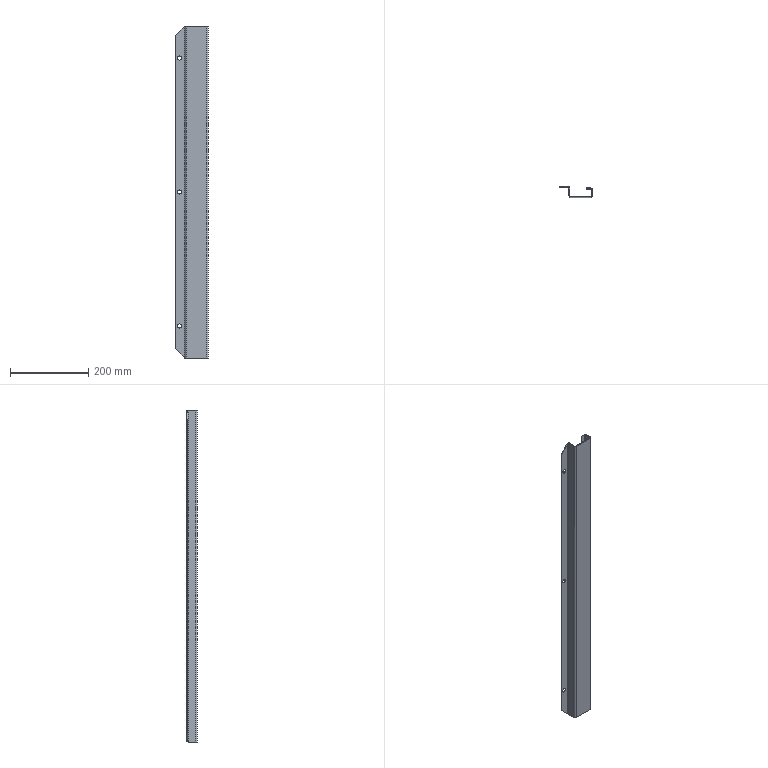Part | STEP file | 750078191 | 1 solid | 32 faces | box 84 x 27 x 850 mm | volume 232667 mm3 | plane 16 | cylinder 14 | spline 2 | commonest cylinder face diameters 10.5 x6 4 x4 8 x4
STEP:
#1=CARTESIAN_POINT('',(-44.,27.,-5.25));
#2=VERTEX_POINT('',#1);
#3=CARTESIAN_POINT('',(-44.,27.,5.25));
#4=VERTEX_POINT('',#3);
#5=CARTESIAN_POINT('',(-44.,27.,0.));
#6=DIRECTION('',(0.,1.,0.));
#7=DIRECTION('',(0.,0.,-1.));
#8=AXIS2_PLACEMENT_3D('',#5,#6,#7);
#9=CIRCLE('',#8,5.25);
#10=EDGE_CURVE('',#2,#4,#9,.T.);
#11=ORIENTED_EDGE('',*,*,#10,.T.);
#12=CARTESIAN_POINT('',(-44.,25.,5.25));
#13=VERTEX_POINT('',#12);
#14=CARTESIAN_POINT('',(-44.,879.567,5.25));
#15=DIRECTION('',(0.,-1.,0.));
#16=VECTOR('',#15,1000.);
#17=LINE('',#14,#16);
#18=EDGE_CURVE('',#4,#13,#17,.T.);
#19=ORIENTED_EDGE('',*,*,#18,.T.);
#20=CARTESIAN_POINT('',(-44.,25.,-5.25));
#21=VERTEX_POINT('',#20);
#22=CARTESIAN_POINT('',(-44.,25.,0.));
#23=DIRECTION('',(0.,1.,0.));
#24=DIRECTION('',(0.,0.,-1.));
#25=AXIS2_PLACEMENT_3D('',#22,#23,#24);
#26=CIRCLE('',#25,5.25);
#27=EDGE_CURVE('',#21,#13,#26,.T.);
#28=ORIENTED_EDGE('',*,*,#27,.F.);
#29=CARTESIAN_POINT('',(-44.,879.567,-5.25));
#30=DIRECTION('',(0.,-1.,0.));
#31=VECTOR('',#30,1000.);
#32=LINE('',#29,#31);
#33=EDGE_CURVE('',#2,#21,#32,.T.);
#34=ORIENTED_EDGE('',*,*,#33,.F.);
#35=EDGE_LOOP('',(#11,#19,#28,#34));
#36=FACE_OUTER_BOUND('',#35,.T.);
#37=CARTESIAN_POINT('',(-44.,879.567,0.));
#38=DIRECTION('',(0.,-1.,0.));
#39=DIRECTION('',(0.,0.,-1.));
#40=AXIS2_PLACEMENT_3D('',#37,#38,#39);
#41=CYLINDRICAL_SURFACE('',#40,5.25);
#42=ADVANCED_FACE('',(#36),#41,.F.);
#43=CARTESIAN_POINT('',(-44.,27.,-348.25));
#44=VERTEX_POINT('',#43);
#45=CARTESIAN_POINT('',(-44.,27.,-337.75));
#46=VERTEX_POINT('',#45);
#47=CARTESIAN_POINT('',(-44.,27.,-343.));
#48=DIRECTION('',(0.,1.,0.));
#49=DIRECTION('',(0.,0.,-1.));
#50=AXIS2_PLACEMENT_3D('',#47,#48,#49);
#51=CIRCLE('',#50,5.25);
#52=EDGE_CURVE('',#44,#46,#51,.T.);
#53=ORIENTED_EDGE('',*,*,#52,.T.);
#54=CARTESIAN_POINT('',(-44.,25.,-337.75));
#55=VERTEX_POINT('',#54);
#56=CARTESIAN_POINT('',(-44.,879.567,-337.75));
#57=DIRECTION('',(0.,-1.,0.));
#58=VECTOR('',#57,1000.);
#59=LINE('',#56,#58);
#60=EDGE_CURVE('',#46,#55,#59,.T.);
#61=ORIENTED_EDGE('',*,*,#60,.T.);
#62=CARTESIAN_POINT('',(-44.,25.,-348.25));
#63=VERTEX_POINT('',#62);
#64=CARTESIAN_POINT('',(-44.,25.,-343.));
#65=DIRECTION('',(0.,1.,0.));
#66=DIRECTION('',(0.,0.,-1.));
#67=AXIS2_PLACEMENT_3D('',#64,#65,#66);
#68=CIRCLE('',#67,5.25);
#69=EDGE_CURVE('',#63,#55,#68,.T.);
#70=ORIENTED_EDGE('',*,*,#69,.F.);
#71=CARTESIAN_POINT('',(-44.,879.567,-348.25));
#72=DIRECTION('',(0.,-1.,0.));
#73=VECTOR('',#72,1000.);
#74=LINE('',#71,#73);
#75=EDGE_CURVE('',#44,#63,#74,.T.);
#76=ORIENTED_EDGE('',*,*,#75,.F.);
#77=EDGE_LOOP('',(#53,#61,#70,#76));
#78=FACE_OUTER_BOUND('',#77,.T.);
#79=CARTESIAN_POINT('',(-44.,879.567,-343.));
#80=DIRECTION('',(0.,-1.,0.));
#81=DIRECTION('',(0.,0.,-1.));
#82=AXIS2_PLACEMENT_3D('',#79,#80,#81);
#83=CYLINDRICAL_SURFACE('',#82,5.25);
#84=ADVANCED_FACE('',(#78),#83,.F.);
#85=CARTESIAN_POINT('',(-44.,27.,337.75));
#86=VERTEX_POINT('',#85);
#87=CARTESIAN_POINT('',(-44.,27.,348.25));
#88=VERTEX_POINT('',#87);
#89=CARTESIAN_POINT('',(-44.,27.,343.));
#90=DIRECTION('',(0.,1.,0.));
#91=DIRECTION('',(0.,0.,-1.));
#92=AXIS2_PLACEMENT_3D('',#89,#90,#91);
#93=CIRCLE('',#92,5.25);
#94=EDGE_CURVE('',#86,#88,#93,.T.);
#95=ORIENTED_EDGE('',*,*,#94,.T.);
#96=CARTESIAN_POINT('',(-44.,25.,348.25));
#97=VERTEX_POINT('',#96);
#98=CARTESIAN_POINT('',(-44.,879.567,348.25));
#99=DIRECTION('',(0.,-1.,0.));
#100=VECTOR('',#99,1000.);
#101=LINE('',#98,#100);
#102=EDGE_CURVE('',#88,#97,#101,.T.);
#103=ORIENTED_EDGE('',*,*,#102,.T.);
#104=CARTESIAN_POINT('',(-44.,25.,337.75));
#105=VERTEX_POINT('',#104);
#106=CARTESIAN_POINT('',(-44.,25.,343.));
#107=DIRECTION('',(0.,1.,0.));
#108=DIRECTION('',(0.,0.,-1.));
#109=AXIS2_PLACEMENT_3D('',#106,#107,#108);
#110=CIRCLE('',#109,5.25);
#111=EDGE_CURVE('',#105,#97,#110,.T.);
#112=ORIENTED_EDGE('',*,*,#111,.F.);
#113=CARTESIAN_POINT('',(-44.,879.567,337.75));
#114=DIRECTION('',(0.,-1.,0.));
#115=VECTOR('',#114,1000.);
#116=LINE('',#113,#115);
#117=EDGE_CURVE('',#86,#105,#116,.T.);
#118=ORIENTED_EDGE('',*,*,#117,.F.);
#119=EDGE_LOOP('',(#95,#103,#112,#118));
#120=FACE_OUTER_BOUND('',#119,.T.);
#121=CARTESIAN_POINT('',(-44.,879.567,343.));
#122=DIRECTION('',(0.,-1.,0.));
#123=DIRECTION('',(0.,0.,-1.));
#124=AXIS2_PLACEMENT_3D('',#121,#122,#123);
#125=CYLINDRICAL_SURFACE('',#124,5.25);
#126=ADVANCED_FACE('',(#120),#125,.F.);
#127=CARTESIAN_POINT('',(26.,0.,425.));
#128=VERTEX_POINT('',#127);
#129=CARTESIAN_POINT('',(-26.,0.,425.));
#130=VERTEX_POINT('',#129);
#131=CARTESIAN_POINT('',(30.,0.,425.));
#132=DIRECTION('',(-1.,0.,0.));
#133=VECTOR('',#132,1000.);
#134=LINE('',#131,#133);
#135=EDGE_CURVE('',#128,#130,#134,.T.);
#136=ORIENTED_EDGE('',*,*,#135,.T.);
#137=CARTESIAN_POINT('',(-26.,0.,-425.));
#138=VERTEX_POINT('',#137);
#139=CARTESIAN_POINT('',(-26.,0.,425.));
#140=DIRECTION('',(0.,0.,-1.));
#141=VECTOR('',#140,1000.);
#142=LINE('',#139,#141);
#143=EDGE_CURVE('',#130,#138,#142,.T.);
#144=ORIENTED_EDGE('',*,*,#143,.T.);
#145=CARTESIAN_POINT('',(26.,0.,-425.));
#146=VERTEX_POINT('',#145);
#147=CARTESIAN_POINT('',(30.,0.,-425.));
#148=DIRECTION('',(1.,0.,0.));
#149=VECTOR('',#148,1000.);
#150=LINE('',#147,#149);
#151=EDGE_CURVE('',#138,#146,#150,.T.);
#152=ORIENTED_EDGE('',*,*,#151,.T.);
#153=CARTESIAN_POINT('',(26.,0.,425.));
#154=DIRECTION('',(0.,0.,1.));
#155=VECTOR('',#154,1000.);
#156=LINE('',#153,#155);
#157=EDGE_CURVE('',#146,#128,#156,.T.);
#158=ORIENTED_EDGE('',*,*,#157,.T.);
#159=EDGE_LOOP('',(#136,#144,#152,#158));
#160=FACE_OUTER_BOUND('',#159,.T.);
#161=CARTESIAN_POINT('',(30.,0.,425.));
#162=DIRECTION('',(0.,-1.,0.));
#163=DIRECTION('',(1.,0.,0.));
#164=AXIS2_PLACEMENT_3D('',#161,#162,#163);
#165=PLANE('',#164);
#166=ADVANCED_FACE('',(#160),#165,.T.);
#167=CARTESIAN_POINT('',(-30.,4.,425.));
#168=VERTEX_POINT('',#167);
#169=CARTESIAN_POINT('',(-26.,4.,425.));
#170=DIRECTION('',(0.,0.,-1.));
#171=DIRECTION('',(-1.,0.,0.));
#172=AXIS2_PLACEMENT_3D('',#169,#170,#171);
#173=CIRCLE('',#172,4.);
#174=EDGE_CURVE('',#130,#168,#173,.T.);
#175=ORIENTED_EDGE('',*,*,#174,.T.);
#176=CARTESIAN_POINT('',(-30.,4.,-425.));
#177=VERTEX_POINT('',#176);
#178=CARTESIAN_POINT('',(-30.,4.,425.));
#179=DIRECTION('',(0.,0.,-1.));
#180=VECTOR('',#179,1000.);
#181=LINE('',#178,#180);
#182=EDGE_CURVE('',#168,#177,#181,.T.);
#183=ORIENTED_EDGE('',*,*,#182,.T.);
#184=CARTESIAN_POINT('',(-26.,4.,-425.));
#185=DIRECTION('',(0.,0.,1.));
#186=DIRECTION('',(-1.,0.,0.));
#187=AXIS2_PLACEMENT_3D('',#184,#185,#186);
#188=CIRCLE('',#187,4.);
#189=EDGE_CURVE('',#177,#138,#188,.T.);
#190=ORIENTED_EDGE('',*,*,#189,.T.);
#191=ORIENTED_EDGE('',*,*,#143,.F.);
#192=EDGE_LOOP('',(#175,#183,#190,#191));
#193=FACE_OUTER_BOUND('',#192,.T.);
#194=CARTESIAN_POINT('',(-26.,4.,425.));
#195=DIRECTION('',(0.,0.,-1.));
#196=DIRECTION('',(-1.,0.,0.));
#197=AXIS2_PLACEMENT_3D('',#194,#195,#196);
#198=CYLINDRICAL_SURFACE('',#197,4.);
#199=ADVANCED_FACE('',(#193),#198,.T.);
#200=CARTESIAN_POINT('',(26.,2.,425.));
#201=VERTEX_POINT('',#200);
#202=CARTESIAN_POINT('',(-26.,2.,425.));
#203=VERTEX_POINT('',#202);
#204=CARTESIAN_POINT('',(-30.,2.,425.));
#205=DIRECTION('',(-1.,0.,0.));
#206=VECTOR('',#205,1000.);
#207=LINE('',#204,#206);
#208=EDGE_CURVE('',#201,#203,#207,.T.);
#209=ORIENTED_EDGE('',*,*,#208,.T.);
#210=CARTESIAN_POINT('',(-28.,4.,425.));
#211=VERTEX_POINT('',#210);
#212=CARTESIAN_POINT('',(-26.,4.,425.));
#213=DIRECTION('',(0.,0.,-1.));
#214=DIRECTION('',(-1.,0.,0.));
#215=AXIS2_PLACEMENT_3D('',#212,#213,#214);
#216=CIRCLE('',#215,2.);
#217=EDGE_CURVE('',#203,#211,#216,.T.);
#218=ORIENTED_EDGE('',*,*,#217,.T.);
#219=CARTESIAN_POINT('',(-28.,23.,425.));
#220=VERTEX_POINT('',#219);
#221=CARTESIAN_POINT('',(-28.,25.,425.));
#222=DIRECTION('',(0.,1.,0.));
#223=VECTOR('',#222,1000.);
#224=LINE('',#221,#223);
#225=EDGE_CURVE('',#211,#220,#224,.T.);
#226=ORIENTED_EDGE('',*,*,#225,.T.);
#227=CARTESIAN_POINT('',(-30.,23.,425.));
#228=VERTEX_POINT('',#227);
#229=CARTESIAN_POINT('',(-30.,23.,425.));
#230=DIRECTION('',(-1.,0.,0.));
#231=VECTOR('',#230,1000.);
#232=LINE('',#229,#231);
#233=EDGE_CURVE('',#220,#228,#232,.T.);
#234=ORIENTED_EDGE('',*,*,#233,.T.);
#235=CARTESIAN_POINT('',(-30.,25.,425.));
#236=DIRECTION('',(0.,-1.,0.));
#237=VECTOR('',#236,1000.);
#238=LINE('',#235,#237);
#239=EDGE_CURVE('',#228,#168,#238,.T.);
#240=ORIENTED_EDGE('',*,*,#239,.T.);
#241=ORIENTED_EDGE('',*,*,#174,.F.);
#242=ORIENTED_EDGE('',*,*,#135,.F.);
#243=CARTESIAN_POINT('',(30.,4.,425.));
#244=VERTEX_POINT('',#243);
#245=CARTESIAN_POINT('',(26.,4.,425.));
#246=DIRECTION('',(0.,0.,1.));
#247=DIRECTION('',(-1.,0.,0.));
#248=AXIS2_PLACEMENT_3D('',#245,#246,#247);
#249=CIRCLE('',#248,4.);
#250=EDGE_CURVE('',#128,#244,#249,.T.);
#251=ORIENTED_EDGE('',*,*,#250,.T.);
#252=CARTESIAN_POINT('',(30.,19.,425.));
#253=VERTEX_POINT('',#252);
#254=CARTESIAN_POINT('',(30.,25.,425.));
#255=DIRECTION('',(0.,1.,0.));
#256=VECTOR('',#255,1000.);
#257=LINE('',#254,#256);
#258=EDGE_CURVE('',#244,#253,#257,.T.);
#259=ORIENTED_EDGE('',*,*,#258,.T.);
#260=CARTESIAN_POINT('',(26.,23.,425.));
#261=VERTEX_POINT('',#260);
#262=CARTESIAN_POINT('',(26.,19.,425.));
#263=DIRECTION('',(0.,0.,1.));
#264=DIRECTION('',(-1.,0.,0.));
#265=AXIS2_PLACEMENT_3D('',#262,#263,#264);
#266=CIRCLE('',#265,4.);
#267=EDGE_CURVE('',#253,#261,#266,.T.);
#268=ORIENTED_EDGE('',*,*,#267,.T.);
#269=CARTESIAN_POINT('',(15.,23.,425.));
#270=VERTEX_POINT('',#269);
#271=CARTESIAN_POINT('',(-30.,23.,425.));
#272=DIRECTION('',(-1.,0.,0.));
#273=VECTOR('',#272,1000.);
#274=LINE('',#271,#273);
#275=EDGE_CURVE('',#261,#270,#274,.T.);
#276=ORIENTED_EDGE('',*,*,#275,.T.);
#277=CARTESIAN_POINT('',(15.,21.,425.));
#278=VERTEX_POINT('',#277);
#279=CARTESIAN_POINT('',(15.,25.,425.));
#280=DIRECTION('',(0.,-1.,0.));
#281=VECTOR('',#280,1000.);
#282=LINE('',#279,#281);
#283=EDGE_CURVE('',#270,#278,#282,.T.);
#284=ORIENTED_EDGE('',*,*,#283,.T.);
#285=CARTESIAN_POINT('',(26.,21.,425.));
#286=VERTEX_POINT('',#285);
#287=CARTESIAN_POINT('',(-30.,21.,425.));
#288=DIRECTION('',(1.,0.,0.));
#289=VECTOR('',#288,1000.);
#290=LINE('',#287,#289);
#291=EDGE_CURVE('',#278,#286,#290,.T.);
#292=ORIENTED_EDGE('',*,*,#291,.T.);
#293=CARTESIAN_POINT('',(28.,19.,425.));
#294=VERTEX_POINT('',#293);
#295=CARTESIAN_POINT('',(26.,19.,425.));
#296=DIRECTION('',(0.,0.,-1.));
#297=DIRECTION('',(-1.,0.,0.));
#298=AXIS2_PLACEMENT_3D('',#295,#296,#297);
#299=CIRCLE('',#298,2.);
#300=EDGE_CURVE('',#286,#294,#299,.T.);
#301=ORIENTED_EDGE('',*,*,#300,.T.);
#302=CARTESIAN_POINT('',(28.,4.,425.));
#303=VERTEX_POINT('',#302);
#304=CARTESIAN_POINT('',(28.,25.,425.));
#305=DIRECTION('',(0.,-1.,0.));
#306=VECTOR('',#305,1000.);
#307=LINE('',#304,#306);
#308=EDGE_CURVE('',#294,#303,#307,.T.);
#309=ORIENTED_EDGE('',*,*,#308,.T.);
#310=CARTESIAN_POINT('',(26.,4.,425.));
#311=DIRECTION('',(0.,0.,-1.));
#312=DIRECTION('',(-1.,0.,0.));
#313=AXIS2_PLACEMENT_3D('',#310,#311,#312);
#314=CIRCLE('',#313,2.);
#315=EDGE_CURVE('',#303,#201,#314,.T.);
#316=ORIENTED_EDGE('',*,*,#315,.T.);
#317=EDGE_LOOP('',(#209,#218,#226,#234,#240,#241,#242,#251,#259,#268,#276,#284,#292,#301,#309,#316));
#318=FACE_OUTER_BOUND('',#317,.T.);
#319=CARTESIAN_POINT('',(-30.,25.,425.));
#320=DIRECTION('',(0.,0.,1.));
#321=DIRECTION('',(1.,0.,0.));
#322=AXIS2_PLACEMENT_3D('',#319,#320,#321);
#323=PLANE('',#322);
#324=ADVANCED_FACE('',(#318),#323,.T.);
#325=ORIENTED_EDGE('',*,*,#250,.F.);
#326=ORIENTED_EDGE('',*,*,#157,.F.);
#327=CARTESIAN_POINT('',(30.,4.,-425.));
#328=VERTEX_POINT('',#327);
#329=CARTESIAN_POINT('',(26.,4.,-425.));
#330=DIRECTION('',(0.,0.,1.));
#331=DIRECTION('',(-1.,0.,0.));
#332=AXIS2_PLACEMENT_3D('',#329,#330,#331);
#333=CIRCLE('',#332,4.);
#334=EDGE_CURVE('',#146,#328,#333,.T.);
#335=ORIENTED_EDGE('',*,*,#334,.T.);
#336=CARTESIAN_POINT('',(30.,4.,425.));
#337=DIRECTION('',(0.,0.,1.));
#338=VECTOR('',#337,1000.);
#339=LINE('',#336,#338);
#340=EDGE_CURVE('',#328,#244,#339,.T.);
#341=ORIENTED_EDGE('',*,*,#340,.T.);
#342=EDGE_LOOP('',(#325,#326,#335,#341));
#343=FACE_OUTER_BOUND('',#342,.T.);
#344=CARTESIAN_POINT('',(26.,4.,425.));
#345=DIRECTION('',(0.,0.,-1.));
#346=DIRECTION('',(-1.,0.,0.));
#347=AXIS2_PLACEMENT_3D('',#344,#345,#346);
#348=CYLINDRICAL_SURFACE('',#347,4.);
#349=ADVANCED_FACE('',(#343),#348,.T.);
#350=CARTESIAN_POINT('',(-28.,4.,-425.));
#351=VERTEX_POINT('',#350);
#352=CARTESIAN_POINT('',(-28.,23.,-425.));
#353=VERTEX_POINT('',#352);
#354=CARTESIAN_POINT('',(-28.,23.,-425.));
#355=DIRECTION('',(0.,1.,0.));
#356=VECTOR('',#355,1000.);
#357=LINE('',#354,#356);
#358=EDGE_CURVE('',#351,#353,#357,.T.);
#359=ORIENTED_EDGE('',*,*,#358,.F.);
#360=CARTESIAN_POINT('',(-26.,2.,-425.));
#361=VERTEX_POINT('',#360);
#362=CARTESIAN_POINT('',(-26.,4.,-425.));
#363=DIRECTION('',(0.,0.,-1.));
#364=DIRECTION('',(-1.,0.,0.));
#365=AXIS2_PLACEMENT_3D('',#362,#363,#364);
#366=CIRCLE('',#365,2.);
#367=EDGE_CURVE('',#361,#351,#366,.T.);
#368=ORIENTED_EDGE('',*,*,#367,.F.);
#369=CARTESIAN_POINT('',(26.,2.,-425.));
#370=VERTEX_POINT('',#369);
#371=CARTESIAN_POINT('',(15.,2.,-425.));
#372=DIRECTION('',(-1.,0.,0.));
#373=VECTOR('',#372,1000.);
#374=LINE('',#371,#373);
#375=EDGE_CURVE('',#370,#361,#374,.T.);
#376=ORIENTED_EDGE('',*,*,#375,.F.);
#377=CARTESIAN_POINT('',(28.,4.,-425.));
#378=VERTEX_POINT('',#377);
#379=CARTESIAN_POINT('',(26.,4.,-425.));
#380=DIRECTION('',(0.,0.,-1.));
#381=DIRECTION('',(-1.,0.,0.));
#382=AXIS2_PLACEMENT_3D('',#379,#380,#381);
#383=CIRCLE('',#382,2.);
#384=EDGE_CURVE('',#378,#370,#383,.T.);
#385=ORIENTED_EDGE('',*,*,#384,.F.);
#386=CARTESIAN_POINT('',(28.,19.,-425.));
#387=VERTEX_POINT('',#386);
#388=CARTESIAN_POINT('',(28.,23.,-425.));
#389=DIRECTION('',(0.,-1.,0.));
#390=VECTOR('',#389,1000.);
#391=LINE('',#388,#390);
#392=EDGE_CURVE('',#387,#378,#391,.T.);
#393=ORIENTED_EDGE('',*,*,#392,.F.);
#394=CARTESIAN_POINT('',(26.,21.,-425.));
#395=VERTEX_POINT('',#394);
#396=CARTESIAN_POINT('',(26.,19.,-425.));
#397=DIRECTION('',(0.,0.,-1.));
#398=DIRECTION('',(-1.,0.,0.));
#399=AXIS2_PLACEMENT_3D('',#396,#397,#398);
#400=CIRCLE('',#399,2.);
#401=EDGE_CURVE('',#395,#387,#400,.T.);
#402=ORIENTED_EDGE('',*,*,#401,.F.);
#403=CARTESIAN_POINT('',(15.,21.,-425.));
#404=VERTEX_POINT('',#403);
#405=CARTESIAN_POINT('',(15.,21.,-425.));
#406=DIRECTION('',(1.,0.,0.));
#407=VECTOR('',#406,1000.);
#408=LINE('',#405,#407);
#409=EDGE_CURVE('',#404,#395,#408,.T.);
#410=ORIENTED_EDGE('',*,*,#409,.F.);
#411=CARTESIAN_POINT('',(15.,23.,-425.));
#412=VERTEX_POINT('',#411);
#413=CARTESIAN_POINT('',(15.,23.,-425.));
#414=DIRECTION('',(0.,-1.,0.));
#415=VECTOR('',#414,1000.);
#416=LINE('',#413,#415);
#417=EDGE_CURVE('',#412,#404,#416,.T.);
#418=ORIENTED_EDGE('',*,*,#417,.F.);
#419=CARTESIAN_POINT('',(26.,23.,-425.));
#420=VERTEX_POINT('',#419);
#421=CARTESIAN_POINT('',(15.,23.,-425.));
#422=DIRECTION('',(-1.,0.,0.));
#423=VECTOR('',#422,1000.);
#424=LINE('',#421,#423);
#425=EDGE_CURVE('',#420,#412,#424,.T.);
#426=ORIENTED_EDGE('',*,*,#425,.F.);
#427=CARTESIAN_POINT('',(30.,19.,-425.));
#428=VERTEX_POINT('',#427);
#429=CARTESIAN_POINT('',(26.,19.,-425.));
#430=DIRECTION('',(0.,0.,1.));
#431=DIRECTION('',(-1.,0.,0.));
#432=AXIS2_PLACEMENT_3D('',#429,#430,#431);
#433=CIRCLE('',#432,4.);
#434=EDGE_CURVE('',#428,#420,#433,.T.);
#435=ORIENTED_EDGE('',*,*,#434,.F.);
#436=CARTESIAN_POINT('',(30.,23.,-425.));
#437=DIRECTION('',(0.,1.,0.));
#438=VECTOR('',#437,1000.);
#439=LINE('',#436,#438);
#440=EDGE_CURVE('',#328,#428,#439,.T.);
#441=ORIENTED_EDGE('',*,*,#440,.F.);
#442=ORIENTED_EDGE('',*,*,#334,.F.);
#443=ORIENTED_EDGE('',*,*,#151,.F.);
#444=ORIENTED_EDGE('',*,*,#189,.F.);
#445=CARTESIAN_POINT('',(-30.,23.,-425.));
#446=VERTEX_POINT('',#445);
#447=CARTESIAN_POINT('',(-30.,23.,-425.));
#448=DIRECTION('',(0.,-1.,0.));
#449=VECTOR('',#448,1000.);
#450=LINE('',#447,#449);
#451=EDGE_CURVE('',#446,#177,#450,.T.);
#452=ORIENTED_EDGE('',*,*,#451,.F.);
#453=CARTESIAN_POINT('',(15.,23.,-425.));
#454=DIRECTION('',(-1.,0.,0.));
#455=VECTOR('',#454,1000.);
#456=LINE('',#453,#455);
#457=EDGE_CURVE('',#353,#446,#456,.T.);
#458=ORIENTED_EDGE('',*,*,#457,.F.);
#459=EDGE_LOOP('',(#359,#368,#376,#385,#393,#402,#410,#418,#426,#435,#441,#442,#443,#444,#452,#458));
#460=FACE_OUTER_BOUND('',#459,.T.);
#461=CARTESIAN_POINT('',(15.,23.,-425.));
#462=DIRECTION('',(0.,0.,1.));
#463=DIRECTION('',(1.,0.,0.));
#464=AXIS2_PLACEMENT_3D('',#461,#462,#463);
#465=PLANE('',#464);
#466=ADVANCED_FACE('',(#460),#465,.F.);
#467=ORIENTED_EDGE('',*,*,#239,.F.);
#468=CARTESIAN_POINT('',(-30.,23.,425.));
#469=DIRECTION('',(0.,0.,-1.));
#470=VECTOR('',#469,1000.);
#471=LINE('',#468,#470);
#472=EDGE_CURVE('',#228,#446,#471,.T.);
#473=ORIENTED_EDGE('',*,*,#472,.T.);
#474=ORIENTED_EDGE('',*,*,#451,.T.);
#475=ORIENTED_EDGE('',*,*,#182,.F.);
#476=EDGE_LOOP('',(#467,#473,#474,#475));
#477=FACE_OUTER_BOUND('',#476,.T.);
#478=CARTESIAN_POINT('',(-30.,0.,425.));
#479=DIRECTION('',(-1.,0.,0.));
#480=DIRECTION('',(0.,-1.,0.));
#481=AXIS2_PLACEMENT_3D('',#478,#479,#480);
#482=PLANE('',#481);
#483=ADVANCED_FACE('',(#477),#482,.T.);
#484=CARTESIAN_POINT('',(-28.,4.,425.));
#485=DIRECTION('',(0.,0.,-1.));
#486=VECTOR('',#485,1000.);
#487=LINE('',#484,#486);
#488=EDGE_CURVE('',#211,#351,#487,.T.);
#489=ORIENTED_EDGE('',*,*,#488,.F.);
#490=ORIENTED_EDGE('',*,*,#217,.F.);
#491=CARTESIAN_POINT('',(-26.,2.,425.));
#492=DIRECTION('',(0.,0.,1.));
#493=VECTOR('',#492,1000.);
#494=LINE('',#491,#493);
#495=EDGE_CURVE('',#361,#203,#494,.T.);
#496=ORIENTED_EDGE('',*,*,#495,.F.);
#497=ORIENTED_EDGE('',*,*,#367,.T.);
#498=EDGE_LOOP('',(#489,#490,#496,#497));
#499=FACE_OUTER_BOUND('',#498,.T.);
#500=CARTESIAN_POINT('',(-26.,4.,425.));
#501=DIRECTION('',(0.,0.,-1.));
#502=DIRECTION('',(-1.,0.,0.));
#503=AXIS2_PLACEMENT_3D('',#500,#501,#502);
#504=CYLINDRICAL_SURFACE('',#503,2.);
#505=ADVANCED_FACE('',(#499),#504,.F.);
#506=ORIENTED_EDGE('',*,*,#495,.T.);
#507=ORIENTED_EDGE('',*,*,#208,.F.);
#508=CARTESIAN_POINT('',(26.,2.,425.));
#509=DIRECTION('',(0.,0.,1.));
#510=VECTOR('',#509,1000.);
#511=LINE('',#508,#510);
#512=EDGE_CURVE('',#370,#201,#511,.T.);
#513=ORIENTED_EDGE('',*,*,#512,.F.);
#514=ORIENTED_EDGE('',*,*,#375,.T.);
#515=EDGE_LOOP('',(#506,#507,#513,#514));
#516=FACE_OUTER_BOUND('',#515,.T.);
#517=CARTESIAN_POINT('',(30.,2.,425.));
#518=DIRECTION('',(0.,-1.,0.));
#519=DIRECTION('',(1.,0.,0.));
#520=AXIS2_PLACEMENT_3D('',#517,#518,#519);
#521=PLANE('',#520);
#522=ADVANCED_FACE('',(#516),#521,.F.);
#523=ORIENTED_EDGE('',*,*,#512,.T.);
#524=ORIENTED_EDGE('',*,*,#315,.F.);
#525=CARTESIAN_POINT('',(28.,4.,425.));
#526=DIRECTION('',(0.,0.,1.));
#527=VECTOR('',#526,1000.);
#528=LINE('',#525,#527);
#529=EDGE_CURVE('',#378,#303,#528,.T.);
#530=ORIENTED_EDGE('',*,*,#529,.F.);
#531=ORIENTED_EDGE('',*,*,#384,.T.);
#532=EDGE_LOOP('',(#523,#524,#530,#531));
#533=FACE_OUTER_BOUND('',#532,.T.);
#534=CARTESIAN_POINT('',(26.,4.,425.));
#535=DIRECTION('',(0.,0.,-1.));
#536=DIRECTION('',(-1.,0.,0.));
#537=AXIS2_PLACEMENT_3D('',#534,#535,#536);
#538=CYLINDRICAL_SURFACE('',#537,2.);
#539=ADVANCED_FACE('',(#533),#538,.F.);
#540=ORIENTED_EDGE('',*,*,#529,.T.);
#541=ORIENTED_EDGE('',*,*,#308,.F.);
#542=CARTESIAN_POINT('',(28.,19.,425.));
#543=DIRECTION('',(0.,0.,1.));
#544=VECTOR('',#543,1000.);
#545=LINE('',#542,#544);
#546=EDGE_CURVE('',#387,#294,#545,.T.);
#547=ORIENTED_EDGE('',*,*,#546,.F.);
#548=ORIENTED_EDGE('',*,*,#392,.T.);
#549=EDGE_LOOP('',(#540,#541,#547,#548));
#550=FACE_OUTER_BOUND('',#549,.T.);
#551=CARTESIAN_POINT('',(28.,23.,425.));
#552=DIRECTION('',(1.,0.,0.));
#553=DIRECTION('',(0.,1.,0.));
#554=AXIS2_PLACEMENT_3D('',#551,#552,#553);
#555=PLANE('',#554);
#556=ADVANCED_FACE('',(#550),#555,.F.);
#557=ORIENTED_EDGE('',*,*,#546,.T.);
#558=ORIENTED_EDGE('',*,*,#300,.F.);
#559=CARTESIAN_POINT('',(26.,21.,425.));
#560=DIRECTION('',(0.,0.,1.));
#561=VECTOR('',#560,1000.);
#562=LINE('',#559,#561);
#563=EDGE_CURVE('',#395,#286,#562,.T.);
#564=ORIENTED_EDGE('',*,*,#563,.F.);
#565=ORIENTED_EDGE('',*,*,#401,.T.);
#566=EDGE_LOOP('',(#557,#558,#564,#565));
#567=FACE_OUTER_BOUND('',#566,.T.);
#568=CARTESIAN_POINT('',(26.,19.,425.));
#569=DIRECTION('',(0.,0.,-1.));
#570=DIRECTION('',(-1.,0.,0.));
#571=AXIS2_PLACEMENT_3D('',#568,#569,#570);
#572=CYLINDRICAL_SURFACE('',#571,2.);
#573=ADVANCED_FACE('',(#567),#572,.F.);
#574=ORIENTED_EDGE('',*,*,#563,.T.);
#575=ORIENTED_EDGE('',*,*,#291,.F.);
#576=CARTESIAN_POINT('',(15.,21.,425.));
#577=DIRECTION('',(0.,0.,1.));
#578=VECTOR('',#577,1000.);
#579=LINE('',#576,#578);
#580=EDGE_CURVE('',#404,#278,#579,.T.);
#581=ORIENTED_EDGE('',*,*,#580,.F.);
#582=ORIENTED_EDGE('',*,*,#409,.T.);
#583=EDGE_LOOP('',(#574,#575,#581,#582));
#584=FACE_OUTER_BOUND('',#583,.T.);
#585=CARTESIAN_POINT('',(15.,21.,425.));
#586=DIRECTION('',(0.,1.,0.));
#587=DIRECTION('',(0.,0.,1.));
#588=AXIS2_PLACEMENT_3D('',#585,#586,#587);
#589=PLANE('',#588);
#590=ADVANCED_FACE('',(#584),#589,.F.);
#591=ORIENTED_EDGE('',*,*,#283,.F.);
#592=CARTESIAN_POINT('',(15.,23.,425.));
#593=DIRECTION('',(0.,0.,1.));
#594=VECTOR('',#593,1000.);
#595=LINE('',#592,#594);
#596=EDGE_CURVE('',#412,#270,#595,.T.);
#597=ORIENTED_EDGE('',*,*,#596,.F.);
#598=ORIENTED_EDGE('',*,*,#417,.T.);
#599=ORIENTED_EDGE('',*,*,#580,.T.);
#600=EDGE_LOOP('',(#591,#597,#598,#599));
#601=FACE_OUTER_BOUND('',#600,.T.);
#602=CARTESIAN_POINT('',(15.,23.,425.));
#603=DIRECTION('',(1.,0.,0.));
#604=DIRECTION('',(0.,0.,-1.));
#605=AXIS2_PLACEMENT_3D('',#602,#603,#604);
#606=PLANE('',#605);
#607=ADVANCED_FACE('',(#601),#606,.F.);
#608=ORIENTED_EDGE('',*,*,#275,.F.);
#609=CARTESIAN_POINT('',(26.,23.,425.));
#610=DIRECTION('',(0.,0.,-1.));
#611=VECTOR('',#610,1000.);
#612=LINE('',#609,#611);
#613=EDGE_CURVE('',#261,#420,#612,.T.);
#614=ORIENTED_EDGE('',*,*,#613,.T.);
#615=ORIENTED_EDGE('',*,*,#425,.T.);
#616=ORIENTED_EDGE('',*,*,#596,.T.);
#617=EDGE_LOOP('',(#608,#614,#615,#616));
#618=FACE_OUTER_BOUND('',#617,.T.);
#619=CARTESIAN_POINT('',(15.,23.,425.));
#620=DIRECTION('',(0.,1.,0.));
#621=DIRECTION('',(0.,0.,1.));
#622=AXIS2_PLACEMENT_3D('',#619,#620,#621);
#623=PLANE('',#622);
#624=ADVANCED_FACE('',(#618),#623,.T.);
#625=ORIENTED_EDGE('',*,*,#267,.F.);
#626=CARTESIAN_POINT('',(30.,19.,425.));
#627=DIRECTION('',(0.,0.,-1.));
#628=VECTOR('',#627,1000.);
#629=LINE('',#626,#628);
#630=EDGE_CURVE('',#253,#428,#629,.T.);
#631=ORIENTED_EDGE('',*,*,#630,.T.);
#632=ORIENTED_EDGE('',*,*,#434,.T.);
#633=ORIENTED_EDGE('',*,*,#613,.F.);
#634=EDGE_LOOP('',(#625,#631,#632,#633));
#635=FACE_OUTER_BOUND('',#634,.T.);
#636=CARTESIAN_POINT('',(26.,19.,425.));
#637=DIRECTION('',(0.,0.,-1.));
#638=DIRECTION('',(-1.,0.,0.));
#639=AXIS2_PLACEMENT_3D('',#636,#637,#638);
#640=CYLINDRICAL_SURFACE('',#639,4.);
#641=ADVANCED_FACE('',(#635),#640,.T.);
#642=ORIENTED_EDGE('',*,*,#258,.F.);
#643=ORIENTED_EDGE('',*,*,#340,.F.);
#644=ORIENTED_EDGE('',*,*,#440,.T.);
#645=ORIENTED_EDGE('',*,*,#630,.F.);
#646=EDGE_LOOP('',(#642,#643,#644,#645));
#647=FACE_OUTER_BOUND('',#646,.T.);
#648=CARTESIAN_POINT('',(30.,23.,425.));
#649=DIRECTION('',(1.,0.,0.));
#650=DIRECTION('',(0.,1.,0.));
#651=AXIS2_PLACEMENT_3D('',#648,#649,#650);
#652=PLANE('',#651);
#653=ADVANCED_FACE('',(#647),#652,.T.);
#654=ORIENTED_EDGE('',*,*,#233,.F.);
#655=CARTESIAN_POINT('',(-32.,27.,423.));
#656=VERTEX_POINT('',#655);
#657=CARTESIAN_POINT('',(-28.,23.,425.));
#658=CARTESIAN_POINT('',(-28.,25.,425.));
#659=CARTESIAN_POINT('',(-29.333,27.,424.333));
#660=CARTESIAN_POINT('',(-32.,27.,423.));
#661=(BOUNDED_CURVE()B_SPLINE_CURVE(3,(#657,#658,#659,#660),.UNSPECIFIED.,.F.,.F.)B_SPLINE_CURVE_WITH_KNOTS((4,4),(0.,0.006653),.UNSPECIFIED.)CURVE()GEOMETRIC_REPRESENTATION_ITEM()RATIONAL_B_SPLINE_CURVE((1.,0.6667,0.5,0.5))REPRESENTATION_ITEM(''));
#662=EDGE_CURVE('',#220,#656,#661,.T.);
#663=ORIENTED_EDGE('',*,*,#662,.T.);
#664=CARTESIAN_POINT('',(-32.,25.,423.));
#665=VERTEX_POINT('',#664);
#666=CARTESIAN_POINT('',(-32.,26.,423.));
#667=DIRECTION('',(0.,-1.,0.));
#668=VECTOR('',#667,1000.);
#669=LINE('',#666,#668);
#670=EDGE_CURVE('',#656,#665,#669,.T.);
#671=ORIENTED_EDGE('',*,*,#670,.T.);
#672=CARTESIAN_POINT('',(-32.,25.,423.));
#673=CARTESIAN_POINT('',(-30.667,25.,424.333));
#674=CARTESIAN_POINT('',(-30.,24.,425.));
#675=CARTESIAN_POINT('',(-30.,23.,425.));
#676=(BOUNDED_CURVE()B_SPLINE_CURVE(3,(#672,#673,#674,#675),.UNSPECIFIED.,.F.,.F.)B_SPLINE_CURVE_WITH_KNOTS((4,4),(0.,0.003785),.UNSPECIFIED.)CURVE()GEOMETRIC_REPRESENTATION_ITEM()RATIONAL_B_SPLINE_CURVE((0.5,0.5,0.6667,1.))REPRESENTATION_ITEM(''));
#677=EDGE_CURVE('',#665,#228,#676,.T.);
#678=ORIENTED_EDGE('',*,*,#677,.T.);
#679=EDGE_LOOP('',(#654,#663,#671,#678));
#680=FACE_OUTER_BOUND('',#679,.T.);
#681=CARTESIAN_POINT('',(-34.,23.,421.));
#682=CARTESIAN_POINT('',(-34.667,23.,421.));
#683=CARTESIAN_POINT('',(-35.333,23.,421.));
#684=CARTESIAN_POINT('',(-36.,23.,421.));
#685=CARTESIAN_POINT('',(-34.,27.,421.));
#686=CARTESIAN_POINT('',(-34.667,28.333,421.));
#687=CARTESIAN_POINT('',(-35.333,29.667,421.));
#688=CARTESIAN_POINT('',(-36.,31.,421.));
#689=CARTESIAN_POINT('',(-30.,27.,425.));
#690=CARTESIAN_POINT('',(-29.333,28.333,425.));
#691=CARTESIAN_POINT('',(-28.667,29.667,425.));
#692=CARTESIAN_POINT('',(-28.,31.,425.));
#693=CARTESIAN_POINT('',(-30.,23.,425.));
#694=CARTESIAN_POINT('',(-29.333,23.,425.));
#695=CARTESIAN_POINT('',(-28.667,23.,425.));
#696=CARTESIAN_POINT('',(-28.,23.,425.));
#697=CARTESIAN_POINT('',(-30.,19.,425.));
#698=CARTESIAN_POINT('',(-29.333,17.667,425.));
#699=CARTESIAN_POINT('',(-28.667,16.333,425.));
#700=CARTESIAN_POINT('',(-28.,15.,425.));
#701=CARTESIAN_POINT('',(-34.,19.,421.));
#702=CARTESIAN_POINT('',(-34.667,17.667,421.));
#703=CARTESIAN_POINT('',(-35.333,16.333,421.));
#704=CARTESIAN_POINT('',(-36.,15.,421.));
#705=CARTESIAN_POINT('',(-34.,23.,421.));
#706=CARTESIAN_POINT('',(-34.667,23.,421.));
#707=CARTESIAN_POINT('',(-35.333,23.,421.));
#708=CARTESIAN_POINT('',(-36.,23.,421.));
#709=(BOUNDED_SURFACE()B_SPLINE_SURFACE(3,3,((#681,#682,#683,#684),(#685,#686,#687,#688),(#689,#690,#691,#692),(#693,#694,#695,#696),(#697,#698,#699,#700),(#701,#702,#703,#704),(#705,#706,#707,#708)),.UNSPECIFIED.,.T.,.F.,.F.)B_SPLINE_SURFACE_WITH_KNOTS((4,3,4),(4,4),(0.,0.5,1.),(0.,1.),.UNSPECIFIED.)GEOMETRIC_REPRESENTATION_ITEM()RATIONAL_B_SPLINE_SURFACE(((1.,1.,1.,1.),(0.3333,0.3333,0.3333,0.3333),(0.3333,0.3333,0.3333,0.3333),(1.,1.,1.,1.),(0.3333,0.3333,0.3333,0.3333),(0.3333,0.3333,0.3333,0.3333),(1.,1.,1.,1.)))REPRESENTATION_ITEM('')SURFACE());
#710=ADVANCED_FACE('',(#680),#709,.T.);
#711=CARTESIAN_POINT('',(-28.,23.,425.));
#712=DIRECTION('',(0.,0.,-1.));
#713=VECTOR('',#712,1000.);
#714=LINE('',#711,#713);
#715=EDGE_CURVE('',#220,#353,#714,.T.);
#716=ORIENTED_EDGE('',*,*,#715,.F.);
#717=ORIENTED_EDGE('',*,*,#225,.F.);
#718=ORIENTED_EDGE('',*,*,#488,.T.);
#719=ORIENTED_EDGE('',*,*,#358,.T.);
#720=EDGE_LOOP('',(#716,#717,#718,#719));
#721=FACE_OUTER_BOUND('',#720,.T.);
#722=CARTESIAN_POINT('',(-28.,0.,425.));
#723=DIRECTION('',(-1.,0.,0.));
#724=DIRECTION('',(0.,-1.,0.));
#725=AXIS2_PLACEMENT_3D('',#722,#723,#724);
#726=PLANE('',#725);
#727=ADVANCED_FACE('',(#721),#726,.F.);
#728=CARTESIAN_POINT('',(-32.,25.,-423.));
#729=VERTEX_POINT('',#728);
#730=CARTESIAN_POINT('',(-32.,25.,-423.));
#731=CARTESIAN_POINT('',(-30.667,25.,-424.333));
#732=CARTESIAN_POINT('',(-30.,24.,-425.));
#733=CARTESIAN_POINT('',(-30.,23.,-425.));
#734=(BOUNDED_CURVE()B_SPLINE_CURVE(3,(#730,#731,#732,#733),.UNSPECIFIED.,.F.,.F.)B_SPLINE_CURVE_WITH_KNOTS((4,4),(0.,0.003785),.UNSPECIFIED.)CURVE()GEOMETRIC_REPRESENTATION_ITEM()RATIONAL_B_SPLINE_CURVE((0.5,0.5,0.6667,1.))REPRESENTATION_ITEM(''));
#735=EDGE_CURVE('',#729,#446,#734,.T.);
#736=ORIENTED_EDGE('',*,*,#735,.F.);
#737=CARTESIAN_POINT('',(-32.,27.,-423.));
#738=VERTEX_POINT('',#737);
#739=CARTESIAN_POINT('',(-32.,26.,-423.));
#740=DIRECTION('',(0.,-1.,0.));
#741=VECTOR('',#740,1000.);
#742=LINE('',#739,#741);
#743=EDGE_CURVE('',#738,#729,#742,.T.);
#744=ORIENTED_EDGE('',*,*,#743,.F.);
#745=CARTESIAN_POINT('',(-28.,23.,-425.));
#746=CARTESIAN_POINT('',(-28.,25.,-425.));
#747=CARTESIAN_POINT('',(-29.333,27.,-424.333));
#748=CARTESIAN_POINT('',(-32.,27.,-423.));
#749=(BOUNDED_CURVE()B_SPLINE_CURVE(3,(#745,#746,#747,#748),.UNSPECIFIED.,.F.,.F.)B_SPLINE_CURVE_WITH_KNOTS((4,4),(0.,0.006696),.UNSPECIFIED.)CURVE()GEOMETRIC_REPRESENTATION_ITEM()RATIONAL_B_SPLINE_CURVE((1.,0.6667,0.5,0.5))REPRESENTATION_ITEM(''));
#750=EDGE_CURVE('',#353,#738,#749,.T.);
#751=ORIENTED_EDGE('',*,*,#750,.F.);
#752=ORIENTED_EDGE('',*,*,#457,.T.);
#753=EDGE_LOOP('',(#736,#744,#751,#752));
#754=FACE_OUTER_BOUND('',#753,.T.);
#755=CARTESIAN_POINT('',(-30.,23.,-425.));
#756=CARTESIAN_POINT('',(-29.333,23.,-425.));
#757=CARTESIAN_POINT('',(-28.667,23.,-425.));
#758=CARTESIAN_POINT('',(-28.,23.,-425.));
#759=CARTESIAN_POINT('',(-30.,19.,-425.));
#760=CARTESIAN_POINT('',(-29.333,17.667,-425.));
#761=CARTESIAN_POINT('',(-28.667,16.333,-425.));
#762=CARTESIAN_POINT('',(-28.,15.,-425.));
#763=CARTESIAN_POINT('',(-34.,19.,-421.));
#764=CARTESIAN_POINT('',(-34.667,17.667,-421.));
#765=CARTESIAN_POINT('',(-35.333,16.333,-421.));
#766=CARTESIAN_POINT('',(-36.,15.,-421.));
#767=CARTESIAN_POINT('',(-34.,23.,-421.));
#768=CARTESIAN_POINT('',(-34.667,23.,-421.));
#769=CARTESIAN_POINT('',(-35.333,23.,-421.));
#770=CARTESIAN_POINT('',(-36.,23.,-421.));
#771=CARTESIAN_POINT('',(-34.,27.,-421.));
#772=CARTESIAN_POINT('',(-34.667,28.333,-421.));
#773=CARTESIAN_POINT('',(-35.333,29.667,-421.));
#774=CARTESIAN_POINT('',(-36.,31.,-421.));
#775=CARTESIAN_POINT('',(-30.,27.,-425.));
#776=CARTESIAN_POINT('',(-29.333,28.333,-425.));
#777=CARTESIAN_POINT('',(-28.667,29.667,-425.));
#778=CARTESIAN_POINT('',(-28.,31.,-425.));
#779=CARTESIAN_POINT('',(-30.,23.,-425.));
#780=CARTESIAN_POINT('',(-29.333,23.,-425.));
#781=CARTESIAN_POINT('',(-28.667,23.,-425.));
#782=CARTESIAN_POINT('',(-28.,23.,-425.));
#783=(BOUNDED_SURFACE()B_SPLINE_SURFACE(3,3,((#755,#756,#757,#758),(#759,#760,#761,#762),(#763,#764,#765,#766),(#767,#768,#769,#770),(#771,#772,#773,#774),(#775,#776,#777,#778),(#779,#780,#781,#782)),.UNSPECIFIED.,.T.,.F.,.F.)B_SPLINE_SURFACE_WITH_KNOTS((4,3,4),(4,4),(0.,0.5,1.),(0.,1.),.UNSPECIFIED.)GEOMETRIC_REPRESENTATION_ITEM()RATIONAL_B_SPLINE_SURFACE(((1.,1.,1.,1.),(0.3333,0.3333,0.3333,0.3333),(0.3333,0.3333,0.3333,0.3333),(1.,1.,1.,1.),(0.3333,0.3333,0.3333,0.3333),(0.3333,0.3333,0.3333,0.3333),(1.,1.,1.,1.)))REPRESENTATION_ITEM('')SURFACE());
#784=ADVANCED_FACE('',(#754),#783,.F.);
#785=CARTESIAN_POINT('',(-32.,25.,425.));
#786=DIRECTION('',(0.,0.,1.));
#787=VECTOR('',#786,1000.);
#788=LINE('',#785,#787);
#789=EDGE_CURVE('',#729,#665,#788,.T.);
#790=ORIENTED_EDGE('',*,*,#789,.F.);
#791=ORIENTED_EDGE('',*,*,#735,.T.);
#792=ORIENTED_EDGE('',*,*,#472,.F.);
#793=ORIENTED_EDGE('',*,*,#677,.F.);
#794=EDGE_LOOP('',(#790,#791,#792,#793));
#795=FACE_OUTER_BOUND('',#794,.T.);
#796=CARTESIAN_POINT('',(-32.,23.,425.));
#797=DIRECTION('',(0.,0.,-1.));
#798=DIRECTION('',(-1.,0.,0.));
#799=AXIS2_PLACEMENT_3D('',#796,#797,#798);
#800=CYLINDRICAL_SURFACE('',#799,2.);
#801=ADVANCED_FACE('',(#795),#800,.F.);
#802=ORIENTED_EDGE('',*,*,#715,.T.);
#803=ORIENTED_EDGE('',*,*,#750,.T.);
#804=CARTESIAN_POINT('',(-32.,27.,425.));
#805=DIRECTION('',(0.,0.,1.));
#806=VECTOR('',#805,1000.);
#807=LINE('',#804,#806);
#808=EDGE_CURVE('',#738,#656,#807,.T.);
#809=ORIENTED_EDGE('',*,*,#808,.T.);
#810=ORIENTED_EDGE('',*,*,#662,.F.);
#811=EDGE_LOOP('',(#802,#803,#809,#810));
#812=FACE_OUTER_BOUND('',#811,.T.);
#813=CARTESIAN_POINT('',(-32.,23.,425.));
#814=DIRECTION('',(0.,0.,-1.));
#815=DIRECTION('',(-1.,0.,0.));
#816=AXIS2_PLACEMENT_3D('',#813,#814,#815);
#817=CYLINDRICAL_SURFACE('',#816,4.);
#818=ADVANCED_FACE('',(#812),#817,.T.);
#819=CARTESIAN_POINT('',(-54.,25.,401.));
#820=VERTEX_POINT('',#819);
#821=CARTESIAN_POINT('',(-54.,27.,401.));
#822=VERTEX_POINT('',#821);
#823=CARTESIAN_POINT('',(-54.,25.,401.));
#824=DIRECTION('',(0.,1.,0.));
#825=VECTOR('',#824,1000.);
#826=LINE('',#823,#825);
#827=EDGE_CURVE('',#820,#822,#826,.T.);
#828=ORIENTED_EDGE('',*,*,#827,.F.);
#829=CARTESIAN_POINT('',(-30.,25.,425.));
#830=DIRECTION('',(-0.7071,0.,-0.7071));
#831=VECTOR('',#830,1000.);
#832=LINE('',#829,#831);
#833=EDGE_CURVE('',#665,#820,#832,.T.);
#834=ORIENTED_EDGE('',*,*,#833,.F.);
#835=ORIENTED_EDGE('',*,*,#670,.F.);
#836=CARTESIAN_POINT('',(-30.,27.,425.));
#837=DIRECTION('',(0.7071,0.,0.7071));
#838=VECTOR('',#837,1000.);
#839=LINE('',#836,#838);
#840=EDGE_CURVE('',#822,#656,#839,.T.);
#841=ORIENTED_EDGE('',*,*,#840,.F.);
#842=EDGE_LOOP('',(#828,#834,#835,#841));
#843=FACE_OUTER_BOUND('',#842,.T.);
#844=CARTESIAN_POINT('',(-30.,25.,425.));
#845=DIRECTION('',(0.7071,0.,-0.7071));
#846=DIRECTION('',(-0.7071,0.,-0.7071));
#847=AXIS2_PLACEMENT_3D('',#844,#845,#846);
#848=PLANE('',#847);
#849=ADVANCED_FACE('',(#843),#848,.F.);
#850=CARTESIAN_POINT('',(-54.,25.,-401.));
#851=VERTEX_POINT('',#850);
#852=CARTESIAN_POINT('',(-455.,25.,0.));
#853=DIRECTION('',(-0.7071,0.,0.7071));
#854=VECTOR('',#853,1000.);
#855=LINE('',#852,#854);
#856=EDGE_CURVE('',#729,#851,#855,.T.);
#857=ORIENTED_EDGE('',*,*,#856,.T.);
#858=CARTESIAN_POINT('',(-54.,27.,-401.));
#859=VERTEX_POINT('',#858);
#860=CARTESIAN_POINT('',(-54.,25.,-401.));
#861=DIRECTION('',(0.,1.,0.));
#862=VECTOR('',#861,1000.);
#863=LINE('',#860,#862);
#864=EDGE_CURVE('',#851,#859,#863,.T.);
#865=ORIENTED_EDGE('',*,*,#864,.T.);
#866=CARTESIAN_POINT('',(-455.,27.,0.));
#867=DIRECTION('',(0.7071,0.,-0.7071));
#868=VECTOR('',#867,1000.);
#869=LINE('',#866,#868);
#870=EDGE_CURVE('',#859,#738,#869,.T.);
#871=ORIENTED_EDGE('',*,*,#870,.T.);
#872=ORIENTED_EDGE('',*,*,#743,.T.);
#873=EDGE_LOOP('',(#857,#865,#871,#872));
#874=FACE_OUTER_BOUND('',#873,.T.);
#875=CARTESIAN_POINT('',(-455.,25.,0.));
#876=DIRECTION('',(-0.7071,0.,-0.7071));
#877=DIRECTION('',(-0.7071,0.,0.7071));
#878=AXIS2_PLACEMENT_3D('',#875,#876,#877);
#879=PLANE('',#878);
#880=ADVANCED_FACE('',(#874),#879,.T.);
#881=ORIENTED_EDGE('',*,*,#856,.F.);
#882=ORIENTED_EDGE('',*,*,#789,.T.);
#883=ORIENTED_EDGE('',*,*,#833,.T.);
#884=CARTESIAN_POINT('',(-54.,25.,425.));
#885=DIRECTION('',(0.,0.,-1.));
#886=VECTOR('',#885,1000.);
#887=LINE('',#884,#886);
#888=EDGE_CURVE('',#820,#851,#887,.T.);
#889=ORIENTED_EDGE('',*,*,#888,.T.);
#890=EDGE_LOOP('',(#881,#882,#883,#889));
#891=FACE_OUTER_BOUND('',#890,.T.);
#892=ORIENTED_EDGE('',*,*,#27,.T.);
#893=CARTESIAN_POINT('',(-44.,25.,0.));
#894=DIRECTION('',(0.,1.,0.));
#895=DIRECTION('',(0.,0.,-1.));
#896=AXIS2_PLACEMENT_3D('',#893,#894,#895);
#897=CIRCLE('',#896,5.25);
#898=EDGE_CURVE('',#13,#21,#897,.T.);
#899=ORIENTED_EDGE('',*,*,#898,.T.);
#900=EDGE_LOOP('',(#892,#899));
#901=FACE_BOUND('',#900,.T.);
#902=ORIENTED_EDGE('',*,*,#69,.T.);
#903=CARTESIAN_POINT('',(-44.,25.,-343.));
#904=DIRECTION('',(0.,1.,0.));
#905=DIRECTION('',(0.,0.,-1.));
#906=AXIS2_PLACEMENT_3D('',#903,#904,#905);
#907=CIRCLE('',#906,5.25);
#908=EDGE_CURVE('',#55,#63,#907,.T.);
#909=ORIENTED_EDGE('',*,*,#908,.T.);
#910=EDGE_LOOP('',(#902,#909));
#911=FACE_BOUND('',#910,.T.);
#912=ORIENTED_EDGE('',*,*,#111,.T.);
#913=CARTESIAN_POINT('',(-44.,25.,343.));
#914=DIRECTION('',(0.,1.,0.));
#915=DIRECTION('',(0.,0.,-1.));
#916=AXIS2_PLACEMENT_3D('',#913,#914,#915);
#917=CIRCLE('',#916,5.25);
#918=EDGE_CURVE('',#97,#105,#917,.T.);
#919=ORIENTED_EDGE('',*,*,#918,.T.);
#920=EDGE_LOOP('',(#912,#919));
#921=FACE_BOUND('',#920,.T.);
#922=CARTESIAN_POINT('',(-30.,25.,425.));
#923=DIRECTION('',(0.,-1.,0.));
#924=DIRECTION('',(1.,0.,0.));
#925=AXIS2_PLACEMENT_3D('',#922,#923,#924);
#926=PLANE('',#925);
#927=ADVANCED_FACE('',(#891,#901,#911,#921),#926,.T.);
#928=ORIENTED_EDGE('',*,*,#840,.T.);
#929=ORIENTED_EDGE('',*,*,#808,.F.);
#930=ORIENTED_EDGE('',*,*,#870,.F.);
#931=CARTESIAN_POINT('',(-54.,27.,425.));
#932=DIRECTION('',(0.,0.,-1.));
#933=VECTOR('',#932,1000.);
#934=LINE('',#931,#933);
#935=EDGE_CURVE('',#822,#859,#934,.T.);
#936=ORIENTED_EDGE('',*,*,#935,.F.);
#937=EDGE_LOOP('',(#928,#929,#930,#936));
#938=FACE_OUTER_BOUND('',#937,.T.);
#939=ORIENTED_EDGE('',*,*,#10,.F.);
#940=CARTESIAN_POINT('',(-44.,27.,0.));
#941=DIRECTION('',(0.,1.,0.));
#942=DIRECTION('',(0.,0.,-1.));
#943=AXIS2_PLACEMENT_3D('',#940,#941,#942);
#944=CIRCLE('',#943,5.25);
#945=EDGE_CURVE('',#4,#2,#944,.T.);
#946=ORIENTED_EDGE('',*,*,#945,.F.);
#947=EDGE_LOOP('',(#939,#946));
#948=FACE_BOUND('',#947,.T.);
#949=ORIENTED_EDGE('',*,*,#52,.F.);
#950=CARTESIAN_POINT('',(-44.,27.,-343.));
#951=DIRECTION('',(0.,1.,0.));
#952=DIRECTION('',(0.,0.,-1.));
#953=AXIS2_PLACEMENT_3D('',#950,#951,#952);
#954=CIRCLE('',#953,5.25);
#955=EDGE_CURVE('',#46,#44,#954,.T.);
#956=ORIENTED_EDGE('',*,*,#955,.F.);
#957=EDGE_LOOP('',(#949,#956));
#958=FACE_BOUND('',#957,.T.);
#959=ORIENTED_EDGE('',*,*,#94,.F.);
#960=CARTESIAN_POINT('',(-44.,27.,343.));
#961=DIRECTION('',(0.,1.,0.));
#962=DIRECTION('',(0.,0.,-1.));
#963=AXIS2_PLACEMENT_3D('',#960,#961,#962);
#964=CIRCLE('',#963,5.25);
#965=EDGE_CURVE('',#88,#86,#964,.T.);
#966=ORIENTED_EDGE('',*,*,#965,.F.);
#967=EDGE_LOOP('',(#959,#966));
#968=FACE_BOUND('',#967,.T.);
#969=CARTESIAN_POINT('',(-30.,27.,425.));
#970=DIRECTION('',(0.,-1.,0.));
#971=DIRECTION('',(1.,0.,0.));
#972=AXIS2_PLACEMENT_3D('',#969,#970,#971);
#973=PLANE('',#972);
#974=ADVANCED_FACE('',(#938,#948,#958,#968),#973,.F.);
#975=ORIENTED_EDGE('',*,*,#864,.F.);
#976=ORIENTED_EDGE('',*,*,#888,.F.);
#977=ORIENTED_EDGE('',*,*,#827,.T.);
#978=ORIENTED_EDGE('',*,*,#935,.T.);
#979=EDGE_LOOP('',(#975,#976,#977,#978));
#980=FACE_OUTER_BOUND('',#979,.T.);
#981=CARTESIAN_POINT('',(-54.,25.,425.));
#982=DIRECTION('',(-1.,0.,0.));
#983=DIRECTION('',(0.,-1.,0.));
#984=AXIS2_PLACEMENT_3D('',#981,#982,#983);
#985=PLANE('',#984);
#986=ADVANCED_FACE('',(#980),#985,.T.);
#987=ORIENTED_EDGE('',*,*,#18,.F.);
#988=ORIENTED_EDGE('',*,*,#945,.T.);
#989=ORIENTED_EDGE('',*,*,#33,.T.);
#990=ORIENTED_EDGE('',*,*,#898,.F.);
#991=EDGE_LOOP('',(#987,#988,#989,#990));
#992=FACE_OUTER_BOUND('',#991,.T.);
#993=CARTESIAN_POINT('',(-44.,879.567,0.));
#994=DIRECTION('',(0.,-1.,0.));
#995=DIRECTION('',(0.,0.,-1.));
#996=AXIS2_PLACEMENT_3D('',#993,#994,#995);
#997=CYLINDRICAL_SURFACE('',#996,5.25);
#998=ADVANCED_FACE('',(#992),#997,.F.);
#999=ORIENTED_EDGE('',*,*,#60,.F.);
#1000=ORIENTED_EDGE('',*,*,#955,.T.);
#1001=ORIENTED_EDGE('',*,*,#75,.T.);
#1002=ORIENTED_EDGE('',*,*,#908,.F.);
#1003=EDGE_LOOP('',(#999,#1000,#1001,#1002));
#1004=FACE_OUTER_BOUND('',#1003,.T.);
#1005=CARTESIAN_POINT('',(-44.,879.567,-343.));
#1006=DIRECTION('',(0.,-1.,0.));
#1007=DIRECTION('',(0.,0.,-1.));
#1008=AXIS2_PLACEMENT_3D('',#1005,#1006,#1007);
#1009=CYLINDRICAL_SURFACE('',#1008,5.25);
#1010=ADVANCED_FACE('',(#1004),#1009,.F.);
#1011=ORIENTED_EDGE('',*,*,#102,.F.);
#1012=ORIENTED_EDGE('',*,*,#965,.T.);
#1013=ORIENTED_EDGE('',*,*,#117,.T.);
#1014=ORIENTED_EDGE('',*,*,#918,.F.);
#1015=EDGE_LOOP('',(#1011,#1012,#1013,#1014));
#1016=FACE_OUTER_BOUND('',#1015,.T.);
#1017=CARTESIAN_POINT('',(-44.,879.567,343.));
#1018=DIRECTION('',(0.,-1.,0.));
#1019=DIRECTION('',(0.,0.,-1.));
#1020=AXIS2_PLACEMENT_3D('',#1017,#1018,#1019);
#1021=CYLINDRICAL_SURFACE('',#1020,5.25);
#1022=ADVANCED_FACE('',(#1016),#1021,.F.);
#1023=CLOSED_SHELL('',(#42,#84,#126,#166,#199,#324,#349,#466,#483,#505,#522,#539,#556,#573,#590,#607,#624,#641,#653,#710,#727,#784,#801,#818,#849,#880,#927,#974,#986,#998,#1010,#1022));
#1024=MANIFOLD_SOLID_BREP('',#1023);
#1025=CARTESIAN_POINT('',(0.,0.,0.));
#1026=DIRECTION('',(0.,0.,1.));
#1027=DIRECTION('',(1.,0.,0.));
#1028=AXIS2_PLACEMENT_3D('',#1025,#1026,#1027);
#1029=(LENGTH_UNIT()NAMED_UNIT(*)SI_UNIT(.MILLI.,.METRE.));
#1030=UNCERTAINTY_MEASURE_WITH_UNIT(LENGTH_MEASURE(0.00001),#1029,'','');
#1031=(NAMED_UNIT(*)PLANE_ANGLE_UNIT()SI_UNIT($,.RADIAN.));
#1032=(NAMED_UNIT(*)SI_UNIT($,.STERADIAN.)SOLID_ANGLE_UNIT());
#1033=(GEOMETRIC_REPRESENTATION_CONTEXT(3)GLOBAL_UNCERTAINTY_ASSIGNED_CONTEXT((#1030))GLOBAL_UNIT_ASSIGNED_CONTEXT((#1029,#1031,#1032))REPRESENTATION_CONTEXT('',''));
#1034=ADVANCED_BREP_SHAPE_REPRESENTATION('',(#1024,#1028),#1033);